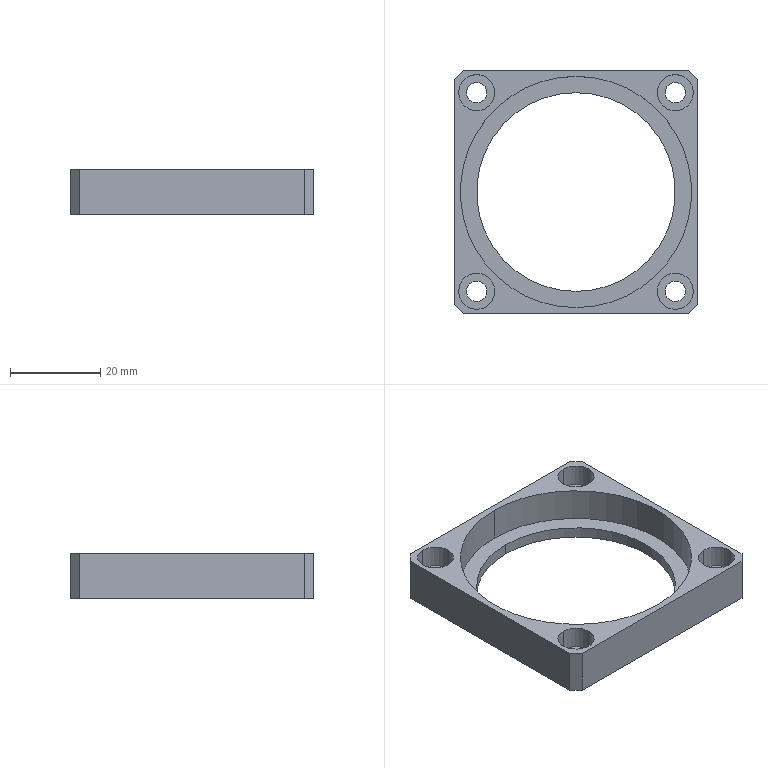Part | NX | 1 solid | 35 faces | box 54 x 54 x 10 mm | volume 8514 mm3 | cylinder 20 | plane 15 | commonest cylinder face diameters 4.5 x8 8 x8 44 x2 51.2 x2
STEP:
#1=CARTESIAN_POINT('',(22.,-18.,-5.));
#2=VERTEX_POINT('',#1);
#3=CARTESIAN_POINT('',(22.,-26.,-5.));
#4=VERTEX_POINT('',#3);
#5=CARTESIAN_POINT('',(22.,-22.,-5.));
#6=DIRECTION('',(0.,0.,1.));
#7=DIRECTION('',(0.,-1.,0.));
#8=AXIS2_PLACEMENT_3D('',#5,#6,#7);
#9=CIRCLE('',#8,4.);
#10=EDGE_CURVE('',#2,#4,#9,.T.);
#11=ORIENTED_EDGE('',*,*,#10,.F.);
#12=CARTESIAN_POINT('',(22.,-18.,0.));
#13=VERTEX_POINT('',#12);
#14=CARTESIAN_POINT('',(22.,-18.,0.));
#15=DIRECTION('',(0.,0.,1.));
#16=VECTOR('',#15,1000.);
#17=LINE('',#14,#16);
#18=EDGE_CURVE('',#13,#2,#17,.F.);
#19=ORIENTED_EDGE('',*,*,#18,.F.);
#20=CARTESIAN_POINT('',(22.,-26.,0.));
#21=VERTEX_POINT('',#20);
#22=CARTESIAN_POINT('',(22.,-22.,0.));
#23=DIRECTION('',(0.,0.,1.));
#24=DIRECTION('',(0.,-1.,0.));
#25=AXIS2_PLACEMENT_3D('',#22,#23,#24);
#26=CIRCLE('',#25,4.);
#27=EDGE_CURVE('',#13,#21,#26,.T.);
#28=ORIENTED_EDGE('',*,*,#27,.T.);
#29=CARTESIAN_POINT('',(22.,-26.,0.));
#30=DIRECTION('',(0.,0.,1.));
#31=VECTOR('',#30,1000.);
#32=LINE('',#29,#31);
#33=EDGE_CURVE('',#21,#4,#32,.F.);
#34=ORIENTED_EDGE('',*,*,#33,.T.);
#35=EDGE_LOOP('',(#11,#19,#28,#34));
#36=FACE_BOUND('',#35,.T.);
#37=CARTESIAN_POINT('',(22.,-22.,0.));
#38=DIRECTION('',(0.,0.,1.));
#39=DIRECTION('',(0.,1.,0.));
#40=AXIS2_PLACEMENT_3D('',#37,#38,#39);
#41=CYLINDRICAL_SURFACE('',#40,4.);
#42=ADVANCED_FACE('',(#36),#41,.F.);
#43=CARTESIAN_POINT('',(22.,-19.75,-10.));
#44=VERTEX_POINT('',#43);
#45=CARTESIAN_POINT('',(22.,-24.25,-10.));
#46=VERTEX_POINT('',#45);
#47=CARTESIAN_POINT('',(22.,-22.,-10.));
#48=DIRECTION('',(0.,0.,1.));
#49=DIRECTION('',(0.,-1.,0.));
#50=AXIS2_PLACEMENT_3D('',#47,#48,#49);
#51=CIRCLE('',#50,2.25);
#52=EDGE_CURVE('',#44,#46,#51,.T.);
#53=ORIENTED_EDGE('',*,*,#52,.F.);
#54=CARTESIAN_POINT('',(22.,-19.75,-5.));
#55=VERTEX_POINT('',#54);
#56=CARTESIAN_POINT('',(22.,-19.75,0.));
#57=DIRECTION('',(0.,0.,1.));
#58=VECTOR('',#57,1000.);
#59=LINE('',#56,#58);
#60=EDGE_CURVE('',#55,#44,#59,.F.);
#61=ORIENTED_EDGE('',*,*,#60,.F.);
#62=CARTESIAN_POINT('',(22.,-24.25,-5.));
#63=VERTEX_POINT('',#62);
#64=CARTESIAN_POINT('',(22.,-22.,-5.));
#65=DIRECTION('',(0.,0.,1.));
#66=DIRECTION('',(0.,-1.,0.));
#67=AXIS2_PLACEMENT_3D('',#64,#65,#66);
#68=CIRCLE('',#67,2.25);
#69=EDGE_CURVE('',#55,#63,#68,.T.);
#70=ORIENTED_EDGE('',*,*,#69,.T.);
#71=CARTESIAN_POINT('',(22.,-24.25,0.));
#72=DIRECTION('',(0.,0.,1.));
#73=VECTOR('',#72,1000.);
#74=LINE('',#71,#73);
#75=EDGE_CURVE('',#63,#46,#74,.F.);
#76=ORIENTED_EDGE('',*,*,#75,.T.);
#77=EDGE_LOOP('',(#53,#61,#70,#76));
#78=FACE_BOUND('',#77,.T.);
#79=CARTESIAN_POINT('',(22.,-22.,0.));
#80=DIRECTION('',(0.,0.,1.));
#81=DIRECTION('',(0.,1.,0.));
#82=AXIS2_PLACEMENT_3D('',#79,#80,#81);
#83=CYLINDRICAL_SURFACE('',#82,2.25);
#84=ADVANCED_FACE('',(#78),#83,.F.);
#85=CARTESIAN_POINT('',(22.,26.,-5.));
#86=VERTEX_POINT('',#85);
#87=CARTESIAN_POINT('',(22.,18.,-5.));
#88=VERTEX_POINT('',#87);
#89=CARTESIAN_POINT('',(22.,22.,-5.));
#90=DIRECTION('',(0.,0.,1.));
#91=DIRECTION('',(0.,-1.,0.));
#92=AXIS2_PLACEMENT_3D('',#89,#90,#91);
#93=CIRCLE('',#92,4.);
#94=EDGE_CURVE('',#86,#88,#93,.T.);
#95=ORIENTED_EDGE('',*,*,#94,.F.);
#96=CARTESIAN_POINT('',(22.,26.,0.));
#97=VERTEX_POINT('',#96);
#98=CARTESIAN_POINT('',(22.,26.,0.));
#99=DIRECTION('',(0.,0.,1.));
#100=VECTOR('',#99,1000.);
#101=LINE('',#98,#100);
#102=EDGE_CURVE('',#97,#86,#101,.F.);
#103=ORIENTED_EDGE('',*,*,#102,.F.);
#104=CARTESIAN_POINT('',(22.,18.,0.));
#105=VERTEX_POINT('',#104);
#106=CARTESIAN_POINT('',(22.,22.,0.));
#107=DIRECTION('',(0.,0.,1.));
#108=DIRECTION('',(0.,-1.,0.));
#109=AXIS2_PLACEMENT_3D('',#106,#107,#108);
#110=CIRCLE('',#109,4.);
#111=EDGE_CURVE('',#97,#105,#110,.T.);
#112=ORIENTED_EDGE('',*,*,#111,.T.);
#113=CARTESIAN_POINT('',(22.,18.,0.));
#114=DIRECTION('',(0.,0.,1.));
#115=VECTOR('',#114,1000.);
#116=LINE('',#113,#115);
#117=EDGE_CURVE('',#105,#88,#116,.F.);
#118=ORIENTED_EDGE('',*,*,#117,.T.);
#119=EDGE_LOOP('',(#95,#103,#112,#118));
#120=FACE_BOUND('',#119,.T.);
#121=CARTESIAN_POINT('',(22.,22.,0.));
#122=DIRECTION('',(0.,0.,1.));
#123=DIRECTION('',(0.,1.,0.));
#124=AXIS2_PLACEMENT_3D('',#121,#122,#123);
#125=CYLINDRICAL_SURFACE('',#124,4.);
#126=ADVANCED_FACE('',(#120),#125,.F.);
#127=CARTESIAN_POINT('',(22.,24.25,-10.));
#128=VERTEX_POINT('',#127);
#129=CARTESIAN_POINT('',(22.,19.75,-10.));
#130=VERTEX_POINT('',#129);
#131=CARTESIAN_POINT('',(22.,22.,-10.));
#132=DIRECTION('',(0.,0.,1.));
#133=DIRECTION('',(0.,-1.,0.));
#134=AXIS2_PLACEMENT_3D('',#131,#132,#133);
#135=CIRCLE('',#134,2.25);
#136=EDGE_CURVE('',#128,#130,#135,.T.);
#137=ORIENTED_EDGE('',*,*,#136,.F.);
#138=CARTESIAN_POINT('',(22.,24.25,-5.));
#139=VERTEX_POINT('',#138);
#140=CARTESIAN_POINT('',(22.,24.25,0.));
#141=DIRECTION('',(0.,0.,1.));
#142=VECTOR('',#141,1000.);
#143=LINE('',#140,#142);
#144=EDGE_CURVE('',#139,#128,#143,.F.);
#145=ORIENTED_EDGE('',*,*,#144,.F.);
#146=CARTESIAN_POINT('',(22.,19.75,-5.));
#147=VERTEX_POINT('',#146);
#148=CARTESIAN_POINT('',(22.,22.,-5.));
#149=DIRECTION('',(0.,0.,1.));
#150=DIRECTION('',(0.,-1.,0.));
#151=AXIS2_PLACEMENT_3D('',#148,#149,#150);
#152=CIRCLE('',#151,2.25);
#153=EDGE_CURVE('',#139,#147,#152,.T.);
#154=ORIENTED_EDGE('',*,*,#153,.T.);
#155=CARTESIAN_POINT('',(22.,19.75,0.));
#156=DIRECTION('',(0.,0.,1.));
#157=VECTOR('',#156,1000.);
#158=LINE('',#155,#157);
#159=EDGE_CURVE('',#147,#130,#158,.F.);
#160=ORIENTED_EDGE('',*,*,#159,.T.);
#161=EDGE_LOOP('',(#137,#145,#154,#160));
#162=FACE_BOUND('',#161,.T.);
#163=CARTESIAN_POINT('',(22.,22.,0.));
#164=DIRECTION('',(0.,0.,1.));
#165=DIRECTION('',(0.,1.,0.));
#166=AXIS2_PLACEMENT_3D('',#163,#164,#165);
#167=CYLINDRICAL_SURFACE('',#166,2.25);
#168=ADVANCED_FACE('',(#162),#167,.F.);
#169=CARTESIAN_POINT('',(-22.,-18.,-5.));
#170=VERTEX_POINT('',#169);
#171=CARTESIAN_POINT('',(-22.,-26.,-5.));
#172=VERTEX_POINT('',#171);
#173=CARTESIAN_POINT('',(-22.,-22.,-5.));
#174=DIRECTION('',(0.,0.,1.));
#175=DIRECTION('',(0.,-1.,0.));
#176=AXIS2_PLACEMENT_3D('',#173,#174,#175);
#177=CIRCLE('',#176,4.);
#178=EDGE_CURVE('',#170,#172,#177,.T.);
#179=ORIENTED_EDGE('',*,*,#178,.F.);
#180=CARTESIAN_POINT('',(-22.,-18.,0.));
#181=VERTEX_POINT('',#180);
#182=CARTESIAN_POINT('',(-22.,-18.,0.));
#183=DIRECTION('',(0.,0.,1.));
#184=VECTOR('',#183,1000.);
#185=LINE('',#182,#184);
#186=EDGE_CURVE('',#181,#170,#185,.F.);
#187=ORIENTED_EDGE('',*,*,#186,.F.);
#188=CARTESIAN_POINT('',(-22.,-26.,0.));
#189=VERTEX_POINT('',#188);
#190=CARTESIAN_POINT('',(-22.,-22.,0.));
#191=DIRECTION('',(0.,0.,1.));
#192=DIRECTION('',(0.,-1.,0.));
#193=AXIS2_PLACEMENT_3D('',#190,#191,#192);
#194=CIRCLE('',#193,4.);
#195=EDGE_CURVE('',#181,#189,#194,.T.);
#196=ORIENTED_EDGE('',*,*,#195,.T.);
#197=CARTESIAN_POINT('',(-22.,-26.,0.));
#198=DIRECTION('',(0.,0.,1.));
#199=VECTOR('',#198,1000.);
#200=LINE('',#197,#199);
#201=EDGE_CURVE('',#189,#172,#200,.F.);
#202=ORIENTED_EDGE('',*,*,#201,.T.);
#203=EDGE_LOOP('',(#179,#187,#196,#202));
#204=FACE_BOUND('',#203,.T.);
#205=CARTESIAN_POINT('',(-22.,-22.,0.));
#206=DIRECTION('',(0.,0.,1.));
#207=DIRECTION('',(0.,1.,0.));
#208=AXIS2_PLACEMENT_3D('',#205,#206,#207);
#209=CYLINDRICAL_SURFACE('',#208,4.);
#210=ADVANCED_FACE('',(#204),#209,.F.);
#211=CARTESIAN_POINT('',(-22.,-19.75,-10.));
#212=VERTEX_POINT('',#211);
#213=CARTESIAN_POINT('',(-22.,-24.25,-10.));
#214=VERTEX_POINT('',#213);
#215=CARTESIAN_POINT('',(-22.,-22.,-10.));
#216=DIRECTION('',(0.,0.,1.));
#217=DIRECTION('',(0.,-1.,0.));
#218=AXIS2_PLACEMENT_3D('',#215,#216,#217);
#219=CIRCLE('',#218,2.25);
#220=EDGE_CURVE('',#212,#214,#219,.T.);
#221=ORIENTED_EDGE('',*,*,#220,.F.);
#222=CARTESIAN_POINT('',(-22.,-19.75,-5.));
#223=VERTEX_POINT('',#222);
#224=CARTESIAN_POINT('',(-22.,-19.75,0.));
#225=DIRECTION('',(0.,0.,1.));
#226=VECTOR('',#225,1000.);
#227=LINE('',#224,#226);
#228=EDGE_CURVE('',#223,#212,#227,.F.);
#229=ORIENTED_EDGE('',*,*,#228,.F.);
#230=CARTESIAN_POINT('',(-22.,-24.25,-5.));
#231=VERTEX_POINT('',#230);
#232=CARTESIAN_POINT('',(-22.,-22.,-5.));
#233=DIRECTION('',(0.,0.,1.));
#234=DIRECTION('',(0.,-1.,0.));
#235=AXIS2_PLACEMENT_3D('',#232,#233,#234);
#236=CIRCLE('',#235,2.25);
#237=EDGE_CURVE('',#223,#231,#236,.T.);
#238=ORIENTED_EDGE('',*,*,#237,.T.);
#239=CARTESIAN_POINT('',(-22.,-24.25,0.));
#240=DIRECTION('',(0.,0.,1.));
#241=VECTOR('',#240,1000.);
#242=LINE('',#239,#241);
#243=EDGE_CURVE('',#231,#214,#242,.F.);
#244=ORIENTED_EDGE('',*,*,#243,.T.);
#245=EDGE_LOOP('',(#221,#229,#238,#244));
#246=FACE_BOUND('',#245,.T.);
#247=CARTESIAN_POINT('',(-22.,-22.,0.));
#248=DIRECTION('',(0.,0.,1.));
#249=DIRECTION('',(0.,1.,0.));
#250=AXIS2_PLACEMENT_3D('',#247,#248,#249);
#251=CYLINDRICAL_SURFACE('',#250,2.25);
#252=ADVANCED_FACE('',(#246),#251,.F.);
#253=CARTESIAN_POINT('',(-22.,26.,-5.));
#254=VERTEX_POINT('',#253);
#255=CARTESIAN_POINT('',(-22.,18.,-5.));
#256=VERTEX_POINT('',#255);
#257=CARTESIAN_POINT('',(-22.,22.,-5.));
#258=DIRECTION('',(0.,0.,1.));
#259=DIRECTION('',(0.,-1.,0.));
#260=AXIS2_PLACEMENT_3D('',#257,#258,#259);
#261=CIRCLE('',#260,4.);
#262=EDGE_CURVE('',#254,#256,#261,.T.);
#263=ORIENTED_EDGE('',*,*,#262,.F.);
#264=CARTESIAN_POINT('',(-22.,26.,0.));
#265=VERTEX_POINT('',#264);
#266=CARTESIAN_POINT('',(-22.,26.,0.));
#267=DIRECTION('',(0.,0.,1.));
#268=VECTOR('',#267,1000.);
#269=LINE('',#266,#268);
#270=EDGE_CURVE('',#265,#254,#269,.F.);
#271=ORIENTED_EDGE('',*,*,#270,.F.);
#272=CARTESIAN_POINT('',(-22.,18.,0.));
#273=VERTEX_POINT('',#272);
#274=CARTESIAN_POINT('',(-22.,22.,0.));
#275=DIRECTION('',(0.,0.,1.));
#276=DIRECTION('',(0.,-1.,0.));
#277=AXIS2_PLACEMENT_3D('',#274,#275,#276);
#278=CIRCLE('',#277,4.);
#279=EDGE_CURVE('',#265,#273,#278,.T.);
#280=ORIENTED_EDGE('',*,*,#279,.T.);
#281=CARTESIAN_POINT('',(-22.,18.,0.));
#282=DIRECTION('',(0.,0.,1.));
#283=VECTOR('',#282,1000.);
#284=LINE('',#281,#283);
#285=EDGE_CURVE('',#273,#256,#284,.F.);
#286=ORIENTED_EDGE('',*,*,#285,.T.);
#287=EDGE_LOOP('',(#263,#271,#280,#286));
#288=FACE_BOUND('',#287,.T.);
#289=CARTESIAN_POINT('',(-22.,22.,0.));
#290=DIRECTION('',(0.,0.,1.));
#291=DIRECTION('',(0.,1.,0.));
#292=AXIS2_PLACEMENT_3D('',#289,#290,#291);
#293=CYLINDRICAL_SURFACE('',#292,4.);
#294=ADVANCED_FACE('',(#288),#293,.F.);
#295=CARTESIAN_POINT('',(-22.,24.25,-10.));
#296=VERTEX_POINT('',#295);
#297=CARTESIAN_POINT('',(-22.,19.75,-10.));
#298=VERTEX_POINT('',#297);
#299=CARTESIAN_POINT('',(-22.,22.,-10.));
#300=DIRECTION('',(0.,0.,1.));
#301=DIRECTION('',(0.,-1.,0.));
#302=AXIS2_PLACEMENT_3D('',#299,#300,#301);
#303=CIRCLE('',#302,2.25);
#304=EDGE_CURVE('',#296,#298,#303,.T.);
#305=ORIENTED_EDGE('',*,*,#304,.F.);
#306=CARTESIAN_POINT('',(-22.,24.25,-5.));
#307=VERTEX_POINT('',#306);
#308=CARTESIAN_POINT('',(-22.,24.25,0.));
#309=DIRECTION('',(0.,0.,1.));
#310=VECTOR('',#309,1000.);
#311=LINE('',#308,#310);
#312=EDGE_CURVE('',#307,#296,#311,.F.);
#313=ORIENTED_EDGE('',*,*,#312,.F.);
#314=CARTESIAN_POINT('',(-22.,19.75,-5.));
#315=VERTEX_POINT('',#314);
#316=CARTESIAN_POINT('',(-22.,22.,-5.));
#317=DIRECTION('',(0.,0.,1.));
#318=DIRECTION('',(0.,-1.,0.));
#319=AXIS2_PLACEMENT_3D('',#316,#317,#318);
#320=CIRCLE('',#319,2.25);
#321=EDGE_CURVE('',#307,#315,#320,.T.);
#322=ORIENTED_EDGE('',*,*,#321,.T.);
#323=CARTESIAN_POINT('',(-22.,19.75,0.));
#324=DIRECTION('',(0.,0.,1.));
#325=VECTOR('',#324,1000.);
#326=LINE('',#323,#325);
#327=EDGE_CURVE('',#315,#298,#326,.F.);
#328=ORIENTED_EDGE('',*,*,#327,.T.);
#329=EDGE_LOOP('',(#305,#313,#322,#328));
#330=FACE_BOUND('',#329,.T.);
#331=CARTESIAN_POINT('',(-22.,22.,0.));
#332=DIRECTION('',(0.,0.,1.));
#333=DIRECTION('',(0.,1.,0.));
#334=AXIS2_PLACEMENT_3D('',#331,#332,#333);
#335=CYLINDRICAL_SURFACE('',#334,2.25);
#336=ADVANCED_FACE('',(#330),#335,.F.);
#337=CARTESIAN_POINT('',(0.,25.6,-7.5));
#338=VERTEX_POINT('',#337);
#339=CARTESIAN_POINT('',(0.,-25.6,-7.5));
#340=VERTEX_POINT('',#339);
#341=CARTESIAN_POINT('',(0.,0.,-7.5));
#342=DIRECTION('',(0.,0.,1.));
#343=DIRECTION('',(0.,-1.,0.));
#344=AXIS2_PLACEMENT_3D('',#341,#342,#343);
#345=CIRCLE('',#344,25.6);
#346=EDGE_CURVE('',#338,#340,#345,.T.);
#347=ORIENTED_EDGE('',*,*,#346,.F.);
#348=CARTESIAN_POINT('',(0.,25.6,0.));
#349=VERTEX_POINT('',#348);
#350=CARTESIAN_POINT('',(0.,25.6,-7.5));
#351=DIRECTION('',(0.,0.,1.));
#352=VECTOR('',#351,1000.);
#353=LINE('',#350,#352);
#354=EDGE_CURVE('',#349,#338,#353,.F.);
#355=ORIENTED_EDGE('',*,*,#354,.F.);
#356=CARTESIAN_POINT('',(0.,-25.6,0.));
#357=VERTEX_POINT('',#356);
#358=CARTESIAN_POINT('',(0.,0.,0.));
#359=DIRECTION('',(0.,0.,1.));
#360=DIRECTION('',(0.,-1.,0.));
#361=AXIS2_PLACEMENT_3D('',#358,#359,#360);
#362=CIRCLE('',#361,25.6);
#363=EDGE_CURVE('',#349,#357,#362,.T.);
#364=ORIENTED_EDGE('',*,*,#363,.T.);
#365=CARTESIAN_POINT('',(0.,-25.6,-7.5));
#366=DIRECTION('',(0.,0.,1.));
#367=VECTOR('',#366,1000.);
#368=LINE('',#365,#367);
#369=EDGE_CURVE('',#357,#340,#368,.F.);
#370=ORIENTED_EDGE('',*,*,#369,.T.);
#371=EDGE_LOOP('',(#347,#355,#364,#370));
#372=FACE_BOUND('',#371,.T.);
#373=CARTESIAN_POINT('',(0.,0.,-7.5));
#374=DIRECTION('',(0.,0.,1.));
#375=DIRECTION('',(0.,1.,0.));
#376=AXIS2_PLACEMENT_3D('',#373,#374,#375);
#377=CYLINDRICAL_SURFACE('',#376,25.6);
#378=ADVANCED_FACE('',(#372),#377,.F.);
#379=CARTESIAN_POINT('',(0.,22.,-7.5));
#380=VERTEX_POINT('',#379);
#381=CARTESIAN_POINT('',(0.,-22.,-7.5));
#382=VERTEX_POINT('',#381);
#383=CARTESIAN_POINT('',(0.,0.,-7.5));
#384=DIRECTION('',(0.,0.,1.));
#385=DIRECTION('',(0.,-1.,0.));
#386=AXIS2_PLACEMENT_3D('',#383,#384,#385);
#387=CIRCLE('',#386,22.);
#388=EDGE_CURVE('',#380,#382,#387,.T.);
#389=ORIENTED_EDGE('',*,*,#388,.T.);
#390=CARTESIAN_POINT('',(0.,-22.,-10.));
#391=VERTEX_POINT('',#390);
#392=CARTESIAN_POINT('',(0.,-22.,0.));
#393=DIRECTION('',(0.,0.,-1.));
#394=VECTOR('',#393,1000.);
#395=LINE('',#392,#394);
#396=EDGE_CURVE('',#391,#382,#395,.F.);
#397=ORIENTED_EDGE('',*,*,#396,.F.);
#398=CARTESIAN_POINT('',(0.,22.,-10.));
#399=VERTEX_POINT('',#398);
#400=CARTESIAN_POINT('',(0.,0.,-10.));
#401=DIRECTION('',(0.,0.,1.));
#402=DIRECTION('',(0.,-1.,0.));
#403=AXIS2_PLACEMENT_3D('',#400,#401,#402);
#404=CIRCLE('',#403,22.);
#405=EDGE_CURVE('',#399,#391,#404,.T.);
#406=ORIENTED_EDGE('',*,*,#405,.F.);
#407=CARTESIAN_POINT('',(0.,22.,0.));
#408=DIRECTION('',(0.,0.,-1.));
#409=VECTOR('',#408,1000.);
#410=LINE('',#407,#409);
#411=EDGE_CURVE('',#399,#380,#410,.F.);
#412=ORIENTED_EDGE('',*,*,#411,.T.);
#413=EDGE_LOOP('',(#389,#397,#406,#412));
#414=FACE_BOUND('',#413,.T.);
#415=CARTESIAN_POINT('',(0.,0.,0.));
#416=DIRECTION('',(0.,0.,-1.));
#417=DIRECTION('',(0.,-1.,0.));
#418=AXIS2_PLACEMENT_3D('',#415,#416,#417);
#419=CYLINDRICAL_SURFACE('',#418,22.);
#420=ADVANCED_FACE('',(#414),#419,.F.);
#421=ORIENTED_EDGE('',*,*,#396,.T.);
#422=CARTESIAN_POINT('',(0.,0.,-7.5));
#423=DIRECTION('',(0.,0.,1.));
#424=DIRECTION('',(0.,-1.,0.));
#425=AXIS2_PLACEMENT_3D('',#422,#423,#424);
#426=CIRCLE('',#425,22.);
#427=EDGE_CURVE('',#382,#380,#426,.T.);
#428=ORIENTED_EDGE('',*,*,#427,.T.);
#429=ORIENTED_EDGE('',*,*,#411,.F.);
#430=CARTESIAN_POINT('',(0.,0.,-10.));
#431=DIRECTION('',(0.,0.,1.));
#432=DIRECTION('',(0.,-1.,0.));
#433=AXIS2_PLACEMENT_3D('',#430,#431,#432);
#434=CIRCLE('',#433,22.);
#435=EDGE_CURVE('',#391,#399,#434,.T.);
#436=ORIENTED_EDGE('',*,*,#435,.F.);
#437=EDGE_LOOP('',(#421,#428,#429,#436));
#438=FACE_BOUND('',#437,.T.);
#439=CARTESIAN_POINT('',(0.,0.,0.));
#440=DIRECTION('',(0.,0.,-1.));
#441=DIRECTION('',(0.,-1.,0.));
#442=AXIS2_PLACEMENT_3D('',#439,#440,#441);
#443=CYLINDRICAL_SURFACE('',#442,22.);
#444=ADVANCED_FACE('',(#438),#443,.F.);
#445=CARTESIAN_POINT('',(22.,-22.,0.));
#446=DIRECTION('',(0.,0.,1.));
#447=DIRECTION('',(0.,-1.,0.));
#448=AXIS2_PLACEMENT_3D('',#445,#446,#447);
#449=CIRCLE('',#448,4.);
#450=EDGE_CURVE('',#21,#13,#449,.T.);
#451=ORIENTED_EDGE('',*,*,#450,.F.);
#452=ORIENTED_EDGE('',*,*,#27,.F.);
#453=EDGE_LOOP('',(#451,#452));
#454=FACE_BOUND('',#453,.T.);
#455=CARTESIAN_POINT('',(22.,22.,0.));
#456=DIRECTION('',(0.,0.,1.));
#457=DIRECTION('',(0.,-1.,0.));
#458=AXIS2_PLACEMENT_3D('',#455,#456,#457);
#459=CIRCLE('',#458,4.);
#460=EDGE_CURVE('',#105,#97,#459,.T.);
#461=ORIENTED_EDGE('',*,*,#460,.F.);
#462=ORIENTED_EDGE('',*,*,#111,.F.);
#463=EDGE_LOOP('',(#461,#462));
#464=FACE_BOUND('',#463,.T.);
#465=CARTESIAN_POINT('',(-22.,-22.,0.));
#466=DIRECTION('',(0.,0.,1.));
#467=DIRECTION('',(0.,-1.,0.));
#468=AXIS2_PLACEMENT_3D('',#465,#466,#467);
#469=CIRCLE('',#468,4.);
#470=EDGE_CURVE('',#189,#181,#469,.T.);
#471=ORIENTED_EDGE('',*,*,#470,.F.);
#472=ORIENTED_EDGE('',*,*,#195,.F.);
#473=EDGE_LOOP('',(#471,#472));
#474=FACE_BOUND('',#473,.T.);
#475=CARTESIAN_POINT('',(-22.,22.,0.));
#476=DIRECTION('',(0.,0.,1.));
#477=DIRECTION('',(0.,-1.,0.));
#478=AXIS2_PLACEMENT_3D('',#475,#476,#477);
#479=CIRCLE('',#478,4.);
#480=EDGE_CURVE('',#273,#265,#479,.T.);
#481=ORIENTED_EDGE('',*,*,#480,.F.);
#482=ORIENTED_EDGE('',*,*,#279,.F.);
#483=EDGE_LOOP('',(#481,#482));
#484=FACE_BOUND('',#483,.T.);
#485=CARTESIAN_POINT('',(0.,0.,0.));
#486=DIRECTION('',(0.,0.,1.));
#487=DIRECTION('',(0.,-1.,0.));
#488=AXIS2_PLACEMENT_3D('',#485,#486,#487);
#489=CIRCLE('',#488,25.6);
#490=EDGE_CURVE('',#357,#349,#489,.T.);
#491=ORIENTED_EDGE('',*,*,#490,.F.);
#492=ORIENTED_EDGE('',*,*,#363,.F.);
#493=EDGE_LOOP('',(#491,#492));
#494=FACE_BOUND('',#493,.T.);
#495=CARTESIAN_POINT('',(27.,-25.,0.));
#496=VERTEX_POINT('',#495);
#497=CARTESIAN_POINT('',(27.,25.,0.));
#498=VERTEX_POINT('',#497);
#499=CARTESIAN_POINT('',(27.,-27.,0.));
#500=DIRECTION('',(0.,1.,0.));
#501=VECTOR('',#500,1000.);
#502=LINE('',#499,#501);
#503=EDGE_CURVE('',#496,#498,#502,.T.);
#504=ORIENTED_EDGE('',*,*,#503,.T.);
#505=CARTESIAN_POINT('',(25.,27.,0.));
#506=VERTEX_POINT('',#505);
#507=CARTESIAN_POINT('',(26.,26.,0.));
#508=DIRECTION('',(-0.7071,0.7071,0.));
#509=VECTOR('',#508,1000.);
#510=LINE('',#507,#509);
#511=EDGE_CURVE('',#498,#506,#510,.T.);
#512=ORIENTED_EDGE('',*,*,#511,.T.);
#513=CARTESIAN_POINT('',(-25.,27.,0.));
#514=VERTEX_POINT('',#513);
#515=CARTESIAN_POINT('',(27.,27.,0.));
#516=DIRECTION('',(-1.,0.,0.));
#517=VECTOR('',#516,1000.);
#518=LINE('',#515,#517);
#519=EDGE_CURVE('',#506,#514,#518,.T.);
#520=ORIENTED_EDGE('',*,*,#519,.T.);
#521=CARTESIAN_POINT('',(-27.,25.,0.));
#522=VERTEX_POINT('',#521);
#523=CARTESIAN_POINT('',(-26.,26.,0.));
#524=DIRECTION('',(-0.7071,-0.7071,0.));
#525=VECTOR('',#524,1000.);
#526=LINE('',#523,#525);
#527=EDGE_CURVE('',#514,#522,#526,.T.);
#528=ORIENTED_EDGE('',*,*,#527,.T.);
#529=CARTESIAN_POINT('',(-27.,-25.,0.));
#530=VERTEX_POINT('',#529);
#531=CARTESIAN_POINT('',(-27.,-27.,0.));
#532=DIRECTION('',(0.,-1.,0.));
#533=VECTOR('',#532,1000.);
#534=LINE('',#531,#533);
#535=EDGE_CURVE('',#522,#530,#534,.T.);
#536=ORIENTED_EDGE('',*,*,#535,.T.);
#537=CARTESIAN_POINT('',(-25.,-27.,0.));
#538=VERTEX_POINT('',#537);
#539=CARTESIAN_POINT('',(-26.,-26.,0.));
#540=DIRECTION('',(0.7071,-0.7071,0.));
#541=VECTOR('',#540,1000.);
#542=LINE('',#539,#541);
#543=EDGE_CURVE('',#530,#538,#542,.T.);
#544=ORIENTED_EDGE('',*,*,#543,.T.);
#545=CARTESIAN_POINT('',(25.,-27.,0.));
#546=VERTEX_POINT('',#545);
#547=CARTESIAN_POINT('',(27.,-27.,0.));
#548=DIRECTION('',(1.,0.,0.));
#549=VECTOR('',#548,1000.);
#550=LINE('',#547,#549);
#551=EDGE_CURVE('',#538,#546,#550,.T.);
#552=ORIENTED_EDGE('',*,*,#551,.T.);
#553=CARTESIAN_POINT('',(26.,-26.,0.));
#554=DIRECTION('',(0.7071,0.7071,0.));
#555=VECTOR('',#554,1000.);
#556=LINE('',#553,#555);
#557=EDGE_CURVE('',#546,#496,#556,.T.);
#558=ORIENTED_EDGE('',*,*,#557,.T.);
#559=EDGE_LOOP('',(#504,#512,#520,#528,#536,#544,#552,#558));
#560=FACE_BOUND('',#559,.T.);
#561=CARTESIAN_POINT('',(0.,0.,0.));
#562=DIRECTION('',(0.,0.,1.));
#563=DIRECTION('',(0.,1.,0.));
#564=AXIS2_PLACEMENT_3D('',#561,#562,#563);
#565=PLANE('',#564);
#566=ADVANCED_FACE('',(#454,#464,#474,#484,#494,#560),#565,.T.);
#567=CARTESIAN_POINT('',(22.,-22.,-10.));
#568=DIRECTION('',(0.,0.,1.));
#569=DIRECTION('',(0.,-1.,0.));
#570=AXIS2_PLACEMENT_3D('',#567,#568,#569);
#571=CIRCLE('',#570,2.25);
#572=EDGE_CURVE('',#46,#44,#571,.T.);
#573=ORIENTED_EDGE('',*,*,#572,.T.);
#574=ORIENTED_EDGE('',*,*,#52,.T.);
#575=EDGE_LOOP('',(#573,#574));
#576=FACE_BOUND('',#575,.T.);
#577=CARTESIAN_POINT('',(22.,22.,-10.));
#578=DIRECTION('',(0.,0.,1.));
#579=DIRECTION('',(0.,-1.,0.));
#580=AXIS2_PLACEMENT_3D('',#577,#578,#579);
#581=CIRCLE('',#580,2.25);
#582=EDGE_CURVE('',#130,#128,#581,.T.);
#583=ORIENTED_EDGE('',*,*,#582,.T.);
#584=ORIENTED_EDGE('',*,*,#136,.T.);
#585=EDGE_LOOP('',(#583,#584));
#586=FACE_BOUND('',#585,.T.);
#587=CARTESIAN_POINT('',(-22.,-22.,-10.));
#588=DIRECTION('',(0.,0.,1.));
#589=DIRECTION('',(0.,-1.,0.));
#590=AXIS2_PLACEMENT_3D('',#587,#588,#589);
#591=CIRCLE('',#590,2.25);
#592=EDGE_CURVE('',#214,#212,#591,.T.);
#593=ORIENTED_EDGE('',*,*,#592,.T.);
#594=ORIENTED_EDGE('',*,*,#220,.T.);
#595=EDGE_LOOP('',(#593,#594));
#596=FACE_BOUND('',#595,.T.);
#597=CARTESIAN_POINT('',(-22.,22.,-10.));
#598=DIRECTION('',(0.,0.,1.));
#599=DIRECTION('',(0.,-1.,0.));
#600=AXIS2_PLACEMENT_3D('',#597,#598,#599);
#601=CIRCLE('',#600,2.25);
#602=EDGE_CURVE('',#298,#296,#601,.T.);
#603=ORIENTED_EDGE('',*,*,#602,.T.);
#604=ORIENTED_EDGE('',*,*,#304,.T.);
#605=EDGE_LOOP('',(#603,#604));
#606=FACE_BOUND('',#605,.T.);
#607=CARTESIAN_POINT('',(25.,27.,-10.));
#608=VERTEX_POINT('',#607);
#609=CARTESIAN_POINT('',(-25.,27.,-10.));
#610=VERTEX_POINT('',#609);
#611=CARTESIAN_POINT('',(27.,27.,-10.));
#612=DIRECTION('',(-1.,0.,0.));
#613=VECTOR('',#612,1000.);
#614=LINE('',#611,#613);
#615=EDGE_CURVE('',#608,#610,#614,.T.);
#616=ORIENTED_EDGE('',*,*,#615,.F.);
#617=CARTESIAN_POINT('',(27.,25.,-10.));
#618=VERTEX_POINT('',#617);
#619=CARTESIAN_POINT('',(25.,27.,-10.));
#620=DIRECTION('',(0.7071,-0.7071,0.));
#621=VECTOR('',#620,1000.);
#622=LINE('',#619,#621);
#623=EDGE_CURVE('',#608,#618,#622,.T.);
#624=ORIENTED_EDGE('',*,*,#623,.T.);
#625=CARTESIAN_POINT('',(27.,-25.,-10.));
#626=VERTEX_POINT('',#625);
#627=CARTESIAN_POINT('',(27.,-27.,-10.));
#628=DIRECTION('',(0.,1.,0.));
#629=VECTOR('',#628,1000.);
#630=LINE('',#627,#629);
#631=EDGE_CURVE('',#626,#618,#630,.T.);
#632=ORIENTED_EDGE('',*,*,#631,.F.);
#633=CARTESIAN_POINT('',(25.,-27.,-10.));
#634=VERTEX_POINT('',#633);
#635=CARTESIAN_POINT('',(27.,-25.,-10.));
#636=DIRECTION('',(-0.7071,-0.7071,0.));
#637=VECTOR('',#636,1000.);
#638=LINE('',#635,#637);
#639=EDGE_CURVE('',#626,#634,#638,.T.);
#640=ORIENTED_EDGE('',*,*,#639,.T.);
#641=CARTESIAN_POINT('',(-25.,-27.,-10.));
#642=VERTEX_POINT('',#641);
#643=CARTESIAN_POINT('',(27.,-27.,-10.));
#644=DIRECTION('',(1.,0.,0.));
#645=VECTOR('',#644,1000.);
#646=LINE('',#643,#645);
#647=EDGE_CURVE('',#642,#634,#646,.T.);
#648=ORIENTED_EDGE('',*,*,#647,.F.);
#649=CARTESIAN_POINT('',(-27.,-25.,-10.));
#650=VERTEX_POINT('',#649);
#651=CARTESIAN_POINT('',(-25.,-27.,-10.));
#652=DIRECTION('',(-0.7071,0.7071,0.));
#653=VECTOR('',#652,1000.);
#654=LINE('',#651,#653);
#655=EDGE_CURVE('',#642,#650,#654,.T.);
#656=ORIENTED_EDGE('',*,*,#655,.T.);
#657=CARTESIAN_POINT('',(-27.,25.,-10.));
#658=VERTEX_POINT('',#657);
#659=CARTESIAN_POINT('',(-27.,-27.,-10.));
#660=DIRECTION('',(0.,-1.,0.));
#661=VECTOR('',#660,1000.);
#662=LINE('',#659,#661);
#663=EDGE_CURVE('',#658,#650,#662,.T.);
#664=ORIENTED_EDGE('',*,*,#663,.F.);
#665=CARTESIAN_POINT('',(-27.,25.,-10.));
#666=DIRECTION('',(0.7071,0.7071,0.));
#667=VECTOR('',#666,1000.);
#668=LINE('',#665,#667);
#669=EDGE_CURVE('',#658,#610,#668,.T.);
#670=ORIENTED_EDGE('',*,*,#669,.T.);
#671=EDGE_LOOP('',(#616,#624,#632,#640,#648,#656,#664,#670));
#672=FACE_BOUND('',#671,.T.);
#673=ORIENTED_EDGE('',*,*,#405,.T.);
#674=ORIENTED_EDGE('',*,*,#435,.T.);
#675=EDGE_LOOP('',(#673,#674));
#676=FACE_BOUND('',#675,.T.);
#677=CARTESIAN_POINT('',(0.,0.,-10.));
#678=DIRECTION('',(0.,0.,1.));
#679=DIRECTION('',(0.,1.,0.));
#680=AXIS2_PLACEMENT_3D('',#677,#678,#679);
#681=PLANE('',#680);
#682=ADVANCED_FACE('',(#576,#586,#596,#606,#672,#676),#681,.F.);
#683=ORIENTED_EDGE('',*,*,#663,.T.);
#684=CARTESIAN_POINT('',(-27.,-25.,0.));
#685=DIRECTION('',(0.,0.,1.));
#686=VECTOR('',#685,1000.);
#687=LINE('',#684,#686);
#688=EDGE_CURVE('',#650,#530,#687,.T.);
#689=ORIENTED_EDGE('',*,*,#688,.T.);
#690=ORIENTED_EDGE('',*,*,#535,.F.);
#691=CARTESIAN_POINT('',(-27.,25.,0.));
#692=DIRECTION('',(0.,0.,-1.));
#693=VECTOR('',#692,1000.);
#694=LINE('',#691,#693);
#695=EDGE_CURVE('',#522,#658,#694,.T.);
#696=ORIENTED_EDGE('',*,*,#695,.T.);
#697=EDGE_LOOP('',(#683,#689,#690,#696));
#698=FACE_BOUND('',#697,.T.);
#699=CARTESIAN_POINT('',(-27.,-27.,0.));
#700=DIRECTION('',(1.,0.,0.));
#701=DIRECTION('',(0.,-1.,0.));
#702=AXIS2_PLACEMENT_3D('',#699,#700,#701);
#703=PLANE('',#702);
#704=ADVANCED_FACE('',(#698),#703,.F.);
#705=ORIENTED_EDGE('',*,*,#647,.T.);
#706=CARTESIAN_POINT('',(25.,-27.,0.));
#707=DIRECTION('',(0.,0.,1.));
#708=VECTOR('',#707,1000.);
#709=LINE('',#706,#708);
#710=EDGE_CURVE('',#634,#546,#709,.T.);
#711=ORIENTED_EDGE('',*,*,#710,.T.);
#712=ORIENTED_EDGE('',*,*,#551,.F.);
#713=CARTESIAN_POINT('',(-25.,-27.,0.));
#714=DIRECTION('',(0.,0.,-1.));
#715=VECTOR('',#714,1000.);
#716=LINE('',#713,#715);
#717=EDGE_CURVE('',#538,#642,#716,.T.);
#718=ORIENTED_EDGE('',*,*,#717,.T.);
#719=EDGE_LOOP('',(#705,#711,#712,#718));
#720=FACE_BOUND('',#719,.T.);
#721=CARTESIAN_POINT('',(27.,-27.,0.));
#722=DIRECTION('',(0.,1.,0.));
#723=DIRECTION('',(1.,0.,0.));
#724=AXIS2_PLACEMENT_3D('',#721,#722,#723);
#725=PLANE('',#724);
#726=ADVANCED_FACE('',(#720),#725,.F.);
#727=ORIENTED_EDGE('',*,*,#631,.T.);
#728=CARTESIAN_POINT('',(27.,25.,0.));
#729=DIRECTION('',(0.,0.,1.));
#730=VECTOR('',#729,1000.);
#731=LINE('',#728,#730);
#732=EDGE_CURVE('',#618,#498,#731,.T.);
#733=ORIENTED_EDGE('',*,*,#732,.T.);
#734=ORIENTED_EDGE('',*,*,#503,.F.);
#735=CARTESIAN_POINT('',(27.,-25.,0.));
#736=DIRECTION('',(0.,0.,-1.));
#737=VECTOR('',#736,1000.);
#738=LINE('',#735,#737);
#739=EDGE_CURVE('',#496,#626,#738,.T.);
#740=ORIENTED_EDGE('',*,*,#739,.T.);
#741=EDGE_LOOP('',(#727,#733,#734,#740));
#742=FACE_BOUND('',#741,.T.);
#743=CARTESIAN_POINT('',(27.,-27.,0.));
#744=DIRECTION('',(-1.,0.,0.));
#745=DIRECTION('',(0.,1.,0.));
#746=AXIS2_PLACEMENT_3D('',#743,#744,#745);
#747=PLANE('',#746);
#748=ADVANCED_FACE('',(#742),#747,.F.);
#749=ORIENTED_EDGE('',*,*,#519,.F.);
#750=CARTESIAN_POINT('',(25.,27.,0.));
#751=DIRECTION('',(0.,0.,-1.));
#752=VECTOR('',#751,1000.);
#753=LINE('',#750,#752);
#754=EDGE_CURVE('',#506,#608,#753,.T.);
#755=ORIENTED_EDGE('',*,*,#754,.T.);
#756=ORIENTED_EDGE('',*,*,#615,.T.);
#757=CARTESIAN_POINT('',(-25.,27.,0.));
#758=DIRECTION('',(0.,0.,1.));
#759=VECTOR('',#758,1000.);
#760=LINE('',#757,#759);
#761=EDGE_CURVE('',#610,#514,#760,.T.);
#762=ORIENTED_EDGE('',*,*,#761,.T.);
#763=EDGE_LOOP('',(#749,#755,#756,#762));
#764=FACE_BOUND('',#763,.T.);
#765=CARTESIAN_POINT('',(27.,27.,0.));
#766=DIRECTION('',(0.,-1.,0.));
#767=DIRECTION('',(-1.,0.,0.));
#768=AXIS2_PLACEMENT_3D('',#765,#766,#767);
#769=PLANE('',#768);
#770=ADVANCED_FACE('',(#764),#769,.F.);
#771=ORIENTED_EDGE('',*,*,#354,.T.);
#772=CARTESIAN_POINT('',(0.,0.,-7.5));
#773=DIRECTION('',(0.,0.,1.));
#774=DIRECTION('',(0.,-1.,0.));
#775=AXIS2_PLACEMENT_3D('',#772,#773,#774);
#776=CIRCLE('',#775,25.6);
#777=EDGE_CURVE('',#340,#338,#776,.T.);
#778=ORIENTED_EDGE('',*,*,#777,.F.);
#779=ORIENTED_EDGE('',*,*,#369,.F.);
#780=ORIENTED_EDGE('',*,*,#490,.T.);
#781=EDGE_LOOP('',(#771,#778,#779,#780));
#782=FACE_BOUND('',#781,.T.);
#783=CARTESIAN_POINT('',(0.,0.,-7.5));
#784=DIRECTION('',(0.,0.,1.));
#785=DIRECTION('',(0.,1.,0.));
#786=AXIS2_PLACEMENT_3D('',#783,#784,#785);
#787=CYLINDRICAL_SURFACE('',#786,25.6);
#788=ADVANCED_FACE('',(#782),#787,.F.);
#789=ORIENTED_EDGE('',*,*,#388,.F.);
#790=ORIENTED_EDGE('',*,*,#427,.F.);
#791=EDGE_LOOP('',(#789,#790));
#792=FACE_BOUND('',#791,.T.);
#793=ORIENTED_EDGE('',*,*,#777,.T.);
#794=ORIENTED_EDGE('',*,*,#346,.T.);
#795=EDGE_LOOP('',(#793,#794));
#796=FACE_BOUND('',#795,.T.);
#797=CARTESIAN_POINT('',(0.,0.,-7.5));
#798=DIRECTION('',(0.,0.,1.));
#799=DIRECTION('',(0.,1.,0.));
#800=AXIS2_PLACEMENT_3D('',#797,#798,#799);
#801=PLANE('',#800);
#802=ADVANCED_FACE('',(#792,#796),#801,.T.);
#803=ORIENTED_EDGE('',*,*,#312,.T.);
#804=ORIENTED_EDGE('',*,*,#602,.F.);
#805=ORIENTED_EDGE('',*,*,#327,.F.);
#806=CARTESIAN_POINT('',(-22.,22.,-5.));
#807=DIRECTION('',(0.,0.,1.));
#808=DIRECTION('',(0.,-1.,0.));
#809=AXIS2_PLACEMENT_3D('',#806,#807,#808);
#810=CIRCLE('',#809,2.25);
#811=EDGE_CURVE('',#315,#307,#810,.T.);
#812=ORIENTED_EDGE('',*,*,#811,.T.);
#813=EDGE_LOOP('',(#803,#804,#805,#812));
#814=FACE_BOUND('',#813,.T.);
#815=CARTESIAN_POINT('',(-22.,22.,0.));
#816=DIRECTION('',(0.,0.,1.));
#817=DIRECTION('',(0.,1.,0.));
#818=AXIS2_PLACEMENT_3D('',#815,#816,#817);
#819=CYLINDRICAL_SURFACE('',#818,2.25);
#820=ADVANCED_FACE('',(#814),#819,.F.);
#821=ORIENTED_EDGE('',*,*,#811,.F.);
#822=ORIENTED_EDGE('',*,*,#321,.F.);
#823=EDGE_LOOP('',(#821,#822));
#824=FACE_BOUND('',#823,.T.);
#825=CARTESIAN_POINT('',(-22.,22.,-5.));
#826=DIRECTION('',(0.,0.,1.));
#827=DIRECTION('',(0.,-1.,0.));
#828=AXIS2_PLACEMENT_3D('',#825,#826,#827);
#829=CIRCLE('',#828,4.);
#830=EDGE_CURVE('',#256,#254,#829,.T.);
#831=ORIENTED_EDGE('',*,*,#830,.T.);
#832=ORIENTED_EDGE('',*,*,#262,.T.);
#833=EDGE_LOOP('',(#831,#832));
#834=FACE_BOUND('',#833,.T.);
#835=CARTESIAN_POINT('',(-19.75,22.,-5.));
#836=DIRECTION('',(0.,0.,-1.));
#837=DIRECTION('',(0.,-1.,0.));
#838=AXIS2_PLACEMENT_3D('',#835,#836,#837);
#839=PLANE('',#838);
#840=ADVANCED_FACE('',(#824,#834),#839,.F.);
#841=ORIENTED_EDGE('',*,*,#270,.T.);
#842=ORIENTED_EDGE('',*,*,#830,.F.);
#843=ORIENTED_EDGE('',*,*,#285,.F.);
#844=ORIENTED_EDGE('',*,*,#480,.T.);
#845=EDGE_LOOP('',(#841,#842,#843,#844));
#846=FACE_BOUND('',#845,.T.);
#847=CARTESIAN_POINT('',(-22.,22.,0.));
#848=DIRECTION('',(0.,0.,1.));
#849=DIRECTION('',(0.,1.,0.));
#850=AXIS2_PLACEMENT_3D('',#847,#848,#849);
#851=CYLINDRICAL_SURFACE('',#850,4.);
#852=ADVANCED_FACE('',(#846),#851,.F.);
#853=ORIENTED_EDGE('',*,*,#228,.T.);
#854=ORIENTED_EDGE('',*,*,#592,.F.);
#855=ORIENTED_EDGE('',*,*,#243,.F.);
#856=CARTESIAN_POINT('',(-22.,-22.,-5.));
#857=DIRECTION('',(0.,0.,1.));
#858=DIRECTION('',(0.,-1.,0.));
#859=AXIS2_PLACEMENT_3D('',#856,#857,#858);
#860=CIRCLE('',#859,2.25);
#861=EDGE_CURVE('',#231,#223,#860,.T.);
#862=ORIENTED_EDGE('',*,*,#861,.T.);
#863=EDGE_LOOP('',(#853,#854,#855,#862));
#864=FACE_BOUND('',#863,.T.);
#865=CARTESIAN_POINT('',(-22.,-22.,0.));
#866=DIRECTION('',(0.,0.,1.));
#867=DIRECTION('',(0.,1.,0.));
#868=AXIS2_PLACEMENT_3D('',#865,#866,#867);
#869=CYLINDRICAL_SURFACE('',#868,2.25);
#870=ADVANCED_FACE('',(#864),#869,.F.);
#871=ORIENTED_EDGE('',*,*,#861,.F.);
#872=ORIENTED_EDGE('',*,*,#237,.F.);
#873=EDGE_LOOP('',(#871,#872));
#874=FACE_BOUND('',#873,.T.);
#875=CARTESIAN_POINT('',(-22.,-22.,-5.));
#876=DIRECTION('',(0.,0.,1.));
#877=DIRECTION('',(0.,-1.,0.));
#878=AXIS2_PLACEMENT_3D('',#875,#876,#877);
#879=CIRCLE('',#878,4.);
#880=EDGE_CURVE('',#172,#170,#879,.T.);
#881=ORIENTED_EDGE('',*,*,#880,.T.);
#882=ORIENTED_EDGE('',*,*,#178,.T.);
#883=EDGE_LOOP('',(#881,#882));
#884=FACE_BOUND('',#883,.T.);
#885=CARTESIAN_POINT('',(-19.75,-22.,-5.));
#886=DIRECTION('',(0.,0.,-1.));
#887=DIRECTION('',(0.,-1.,0.));
#888=AXIS2_PLACEMENT_3D('',#885,#886,#887);
#889=PLANE('',#888);
#890=ADVANCED_FACE('',(#874,#884),#889,.F.);
#891=ORIENTED_EDGE('',*,*,#186,.T.);
#892=ORIENTED_EDGE('',*,*,#880,.F.);
#893=ORIENTED_EDGE('',*,*,#201,.F.);
#894=ORIENTED_EDGE('',*,*,#470,.T.);
#895=EDGE_LOOP('',(#891,#892,#893,#894));
#896=FACE_BOUND('',#895,.T.);
#897=CARTESIAN_POINT('',(-22.,-22.,0.));
#898=DIRECTION('',(0.,0.,1.));
#899=DIRECTION('',(0.,1.,0.));
#900=AXIS2_PLACEMENT_3D('',#897,#898,#899);
#901=CYLINDRICAL_SURFACE('',#900,4.);
#902=ADVANCED_FACE('',(#896),#901,.F.);
#903=ORIENTED_EDGE('',*,*,#144,.T.);
#904=ORIENTED_EDGE('',*,*,#582,.F.);
#905=ORIENTED_EDGE('',*,*,#159,.F.);
#906=CARTESIAN_POINT('',(22.,22.,-5.));
#907=DIRECTION('',(0.,0.,1.));
#908=DIRECTION('',(0.,-1.,0.));
#909=AXIS2_PLACEMENT_3D('',#906,#907,#908);
#910=CIRCLE('',#909,2.25);
#911=EDGE_CURVE('',#147,#139,#910,.T.);
#912=ORIENTED_EDGE('',*,*,#911,.T.);
#913=EDGE_LOOP('',(#903,#904,#905,#912));
#914=FACE_BOUND('',#913,.T.);
#915=CARTESIAN_POINT('',(22.,22.,0.));
#916=DIRECTION('',(0.,0.,1.));
#917=DIRECTION('',(0.,1.,0.));
#918=AXIS2_PLACEMENT_3D('',#915,#916,#917);
#919=CYLINDRICAL_SURFACE('',#918,2.25);
#920=ADVANCED_FACE('',(#914),#919,.F.);
#921=ORIENTED_EDGE('',*,*,#911,.F.);
#922=ORIENTED_EDGE('',*,*,#153,.F.);
#923=EDGE_LOOP('',(#921,#922));
#924=FACE_BOUND('',#923,.T.);
#925=CARTESIAN_POINT('',(22.,22.,-5.));
#926=DIRECTION('',(0.,0.,1.));
#927=DIRECTION('',(0.,-1.,0.));
#928=AXIS2_PLACEMENT_3D('',#925,#926,#927);
#929=CIRCLE('',#928,4.);
#930=EDGE_CURVE('',#88,#86,#929,.T.);
#931=ORIENTED_EDGE('',*,*,#930,.T.);
#932=ORIENTED_EDGE('',*,*,#94,.T.);
#933=EDGE_LOOP('',(#931,#932));
#934=FACE_BOUND('',#933,.T.);
#935=CARTESIAN_POINT('',(24.25,22.,-5.));
#936=DIRECTION('',(0.,0.,-1.));
#937=DIRECTION('',(0.,-1.,0.));
#938=AXIS2_PLACEMENT_3D('',#935,#936,#937);
#939=PLANE('',#938);
#940=ADVANCED_FACE('',(#924,#934),#939,.F.);
#941=ORIENTED_EDGE('',*,*,#102,.T.);
#942=ORIENTED_EDGE('',*,*,#930,.F.);
#943=ORIENTED_EDGE('',*,*,#117,.F.);
#944=ORIENTED_EDGE('',*,*,#460,.T.);
#945=EDGE_LOOP('',(#941,#942,#943,#944));
#946=FACE_BOUND('',#945,.T.);
#947=CARTESIAN_POINT('',(22.,22.,0.));
#948=DIRECTION('',(0.,0.,1.));
#949=DIRECTION('',(0.,1.,0.));
#950=AXIS2_PLACEMENT_3D('',#947,#948,#949);
#951=CYLINDRICAL_SURFACE('',#950,4.);
#952=ADVANCED_FACE('',(#946),#951,.F.);
#953=ORIENTED_EDGE('',*,*,#60,.T.);
#954=ORIENTED_EDGE('',*,*,#572,.F.);
#955=ORIENTED_EDGE('',*,*,#75,.F.);
#956=CARTESIAN_POINT('',(22.,-22.,-5.));
#957=DIRECTION('',(0.,0.,1.));
#958=DIRECTION('',(0.,-1.,0.));
#959=AXIS2_PLACEMENT_3D('',#956,#957,#958);
#960=CIRCLE('',#959,2.25);
#961=EDGE_CURVE('',#63,#55,#960,.T.);
#962=ORIENTED_EDGE('',*,*,#961,.T.);
#963=EDGE_LOOP('',(#953,#954,#955,#962));
#964=FACE_BOUND('',#963,.T.);
#965=CARTESIAN_POINT('',(22.,-22.,0.));
#966=DIRECTION('',(0.,0.,1.));
#967=DIRECTION('',(0.,1.,0.));
#968=AXIS2_PLACEMENT_3D('',#965,#966,#967);
#969=CYLINDRICAL_SURFACE('',#968,2.25);
#970=ADVANCED_FACE('',(#964),#969,.F.);
#971=ORIENTED_EDGE('',*,*,#961,.F.);
#972=ORIENTED_EDGE('',*,*,#69,.F.);
#973=EDGE_LOOP('',(#971,#972));
#974=FACE_BOUND('',#973,.T.);
#975=CARTESIAN_POINT('',(22.,-22.,-5.));
#976=DIRECTION('',(0.,0.,1.));
#977=DIRECTION('',(0.,-1.,0.));
#978=AXIS2_PLACEMENT_3D('',#975,#976,#977);
#979=CIRCLE('',#978,4.);
#980=EDGE_CURVE('',#4,#2,#979,.T.);
#981=ORIENTED_EDGE('',*,*,#980,.T.);
#982=ORIENTED_EDGE('',*,*,#10,.T.);
#983=EDGE_LOOP('',(#981,#982));
#984=FACE_BOUND('',#983,.T.);
#985=CARTESIAN_POINT('',(24.25,-22.,-5.));
#986=DIRECTION('',(0.,0.,-1.));
#987=DIRECTION('',(0.,-1.,0.));
#988=AXIS2_PLACEMENT_3D('',#985,#986,#987);
#989=PLANE('',#988);
#990=ADVANCED_FACE('',(#974,#984),#989,.F.);
#991=ORIENTED_EDGE('',*,*,#18,.T.);
#992=ORIENTED_EDGE('',*,*,#980,.F.);
#993=ORIENTED_EDGE('',*,*,#33,.F.);
#994=ORIENTED_EDGE('',*,*,#450,.T.);
#995=EDGE_LOOP('',(#991,#992,#993,#994));
#996=FACE_BOUND('',#995,.T.);
#997=CARTESIAN_POINT('',(22.,-22.,0.));
#998=DIRECTION('',(0.,0.,1.));
#999=DIRECTION('',(0.,1.,0.));
#1000=AXIS2_PLACEMENT_3D('',#997,#998,#999);
#1001=CYLINDRICAL_SURFACE('',#1000,4.);
#1002=ADVANCED_FACE('',(#996),#1001,.F.);
#1003=ORIENTED_EDGE('',*,*,#511,.F.);
#1004=ORIENTED_EDGE('',*,*,#732,.F.);
#1005=ORIENTED_EDGE('',*,*,#623,.F.);
#1006=ORIENTED_EDGE('',*,*,#754,.F.);
#1007=EDGE_LOOP('',(#1003,#1004,#1005,#1006));
#1008=FACE_BOUND('',#1007,.T.);
#1009=CARTESIAN_POINT('',(25.,27.,0.));
#1010=DIRECTION('',(-0.7071,-0.7071,0.));
#1011=DIRECTION('',(0.,0.,1.));
#1012=AXIS2_PLACEMENT_3D('',#1009,#1010,#1011);
#1013=PLANE('',#1012);
#1014=ADVANCED_FACE('',(#1008),#1013,.F.);
#1015=ORIENTED_EDGE('',*,*,#557,.F.);
#1016=ORIENTED_EDGE('',*,*,#710,.F.);
#1017=ORIENTED_EDGE('',*,*,#639,.F.);
#1018=ORIENTED_EDGE('',*,*,#739,.F.);
#1019=EDGE_LOOP('',(#1015,#1016,#1017,#1018));
#1020=FACE_BOUND('',#1019,.T.);
#1021=CARTESIAN_POINT('',(27.,-25.,0.));
#1022=DIRECTION('',(-0.7071,0.7071,0.));
#1023=DIRECTION('',(0.,0.,1.));
#1024=AXIS2_PLACEMENT_3D('',#1021,#1022,#1023);
#1025=PLANE('',#1024);
#1026=ADVANCED_FACE('',(#1020),#1025,.F.);
#1027=ORIENTED_EDGE('',*,*,#543,.F.);
#1028=ORIENTED_EDGE('',*,*,#688,.F.);
#1029=ORIENTED_EDGE('',*,*,#655,.F.);
#1030=ORIENTED_EDGE('',*,*,#717,.F.);
#1031=EDGE_LOOP('',(#1027,#1028,#1029,#1030));
#1032=FACE_BOUND('',#1031,.T.);
#1033=CARTESIAN_POINT('',(-25.,-27.,0.));
#1034=DIRECTION('',(0.7071,0.7071,0.));
#1035=DIRECTION('',(0.,0.,1.));
#1036=AXIS2_PLACEMENT_3D('',#1033,#1034,#1035);
#1037=PLANE('',#1036);
#1038=ADVANCED_FACE('',(#1032),#1037,.F.);
#1039=ORIENTED_EDGE('',*,*,#527,.F.);
#1040=ORIENTED_EDGE('',*,*,#761,.F.);
#1041=ORIENTED_EDGE('',*,*,#669,.F.);
#1042=ORIENTED_EDGE('',*,*,#695,.F.);
#1043=EDGE_LOOP('',(#1039,#1040,#1041,#1042));
#1044=FACE_BOUND('',#1043,.T.);
#1045=CARTESIAN_POINT('',(-27.,25.,0.));
#1046=DIRECTION('',(0.7071,-0.7071,0.));
#1047=DIRECTION('',(0.,0.,1.));
#1048=AXIS2_PLACEMENT_3D('',#1045,#1046,#1047);
#1049=PLANE('',#1048);
#1050=ADVANCED_FACE('',(#1044),#1049,.F.);
#1051=CLOSED_SHELL('',(#42,#84,#126,#168,#210,#252,#294,#336,#378,#420,#444,#566,#682,#704,#726,#748,#770,#788,#802,#820,#840,#852,#870,#890,#902,#920,#940,#952,#970,#990,#1002,#1014,#1026,#1038,#1050));
#1052=MANIFOLD_SOLID_BREP('',#1051);
#1053=(LENGTH_UNIT()NAMED_UNIT(*)SI_UNIT(.MILLI.,.METRE.));
#1054=UNCERTAINTY_MEASURE_WITH_UNIT(LENGTH_MEASURE(0.00001),#1053,'','');
#1055=(NAMED_UNIT(*)PLANE_ANGLE_UNIT()SI_UNIT($,.RADIAN.));
#1056=(NAMED_UNIT(*)SI_UNIT($,.STERADIAN.)SOLID_ANGLE_UNIT());
#1057=(GEOMETRIC_REPRESENTATION_CONTEXT(3)GLOBAL_UNCERTAINTY_ASSIGNED_CONTEXT((#1054))GLOBAL_UNIT_ASSIGNED_CONTEXT((#1053,#1055,#1056))REPRESENTATION_CONTEXT('',''));
#1058=ADVANCED_BREP_SHAPE_REPRESENTATION('',(#1052),#1057);